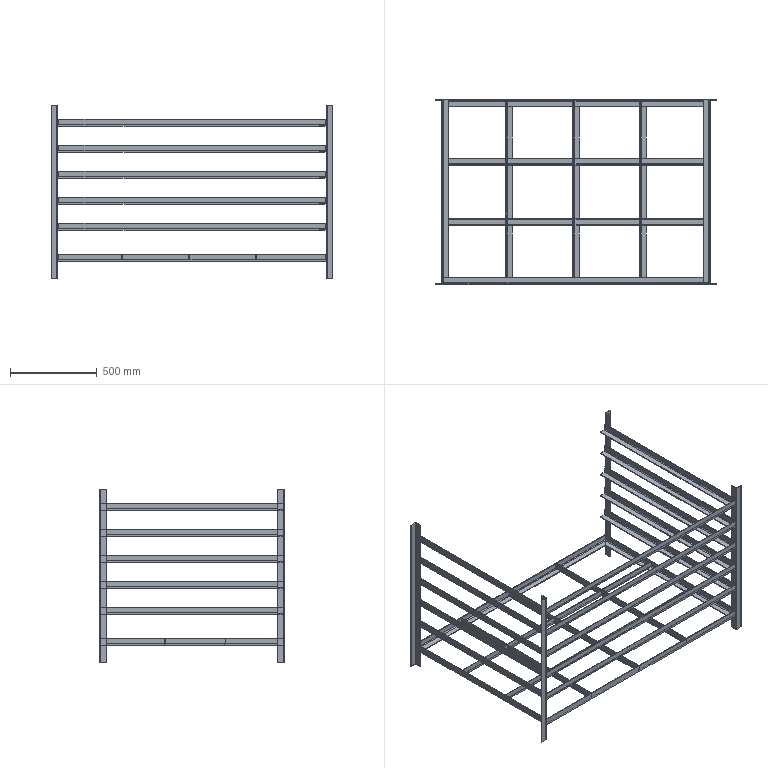Part | SolidWorks | features 3DProfileFeature 1, WeldMemberFeat 1, WeldmentFeature 1 | 34 solids | 452 faces | box 1629 x 1070 x 1000 mm | volume 10278361 mm3 | plane 350 | cylinder 102 | commonest cylinder face diameters 2.667 x68 10 x34